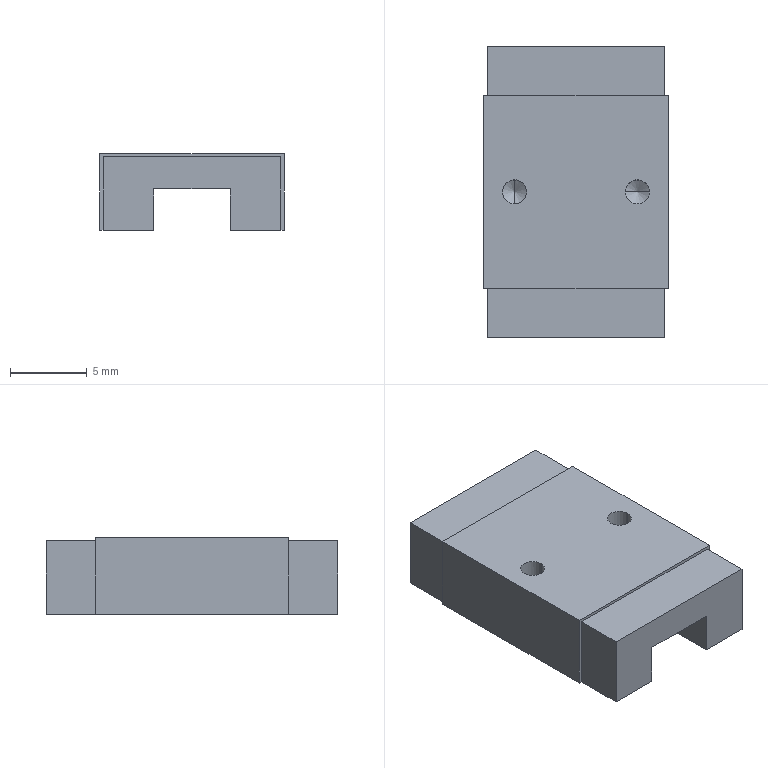Part | SolidWorks | features BaseBody 1 | 1 solid | 26 faces | box 12 x 19 x 5 mm | volume 849.461 mm3 | plane 18 | cylinder 4 | cone 4 | commonest cylinder face diameters 1.567 x4
STEP:
#1=CARTESIAN_POINT('',(-40.025,3.878,3.5));
#2=VERTEX_POINT('',#1);
#3=CARTESIAN_POINT('',(-39.242,3.095,3.5));
#4=VERTEX_POINT('',#3);
#5=CARTESIAN_POINT('',(-39.242,3.878,3.5));
#6=DIRECTION('',(0.,0.,1.));
#7=DIRECTION('',(1.,0.,0.));
#8=AXIS2_PLACEMENT_3D('',#5,#6,#7);
#9=CIRCLE('',#8,0.7835);
#10=EDGE_CURVE('',#2,#4,#9,.T.);
#11=ORIENTED_EDGE('',*,*,#10,.F.);
#12=CARTESIAN_POINT('',(-40.025,3.878,5.));
#13=VERTEX_POINT('',#12);
#14=CARTESIAN_POINT('',(-40.025,3.878,4.25));
#15=DIRECTION('',(0.,0.,1.));
#16=VECTOR('',#15,1000.);
#17=LINE('',#14,#16);
#18=EDGE_CURVE('',#2,#13,#17,.T.);
#19=ORIENTED_EDGE('',*,*,#18,.T.);
#20=CARTESIAN_POINT('',(-38.458,3.878,5.));
#21=VERTEX_POINT('',#20);
#22=CARTESIAN_POINT('',(-39.242,3.878,5.));
#23=DIRECTION('',(0.,0.,-1.));
#24=DIRECTION('',(1.,0.,0.));
#25=AXIS2_PLACEMENT_3D('',#22,#23,#24);
#26=CIRCLE('',#25,0.7835);
#27=EDGE_CURVE('',#21,#13,#26,.T.);
#28=ORIENTED_EDGE('',*,*,#27,.F.);
#29=CARTESIAN_POINT('',(-38.458,3.878,3.5));
#30=VERTEX_POINT('',#29);
#31=CARTESIAN_POINT('',(-38.458,3.878,4.25));
#32=DIRECTION('',(0.,0.,1.));
#33=VECTOR('',#32,1000.);
#34=LINE('',#31,#33);
#35=EDGE_CURVE('',#30,#21,#34,.T.);
#36=ORIENTED_EDGE('',*,*,#35,.F.);
#37=CARTESIAN_POINT('',(-39.242,3.878,3.5));
#38=DIRECTION('',(0.,0.,1.));
#39=DIRECTION('',(1.,0.,0.));
#40=AXIS2_PLACEMENT_3D('',#37,#38,#39);
#41=CIRCLE('',#40,0.7835);
#42=EDGE_CURVE('',#4,#30,#41,.T.);
#43=ORIENTED_EDGE('',*,*,#42,.F.);
#44=EDGE_LOOP('',(#11,#19,#28,#36,#43));
#45=FACE_OUTER_BOUND('',#44,.T.);
#46=CARTESIAN_POINT('',(-39.242,3.878,4.25));
#47=DIRECTION('',(0.,0.,1.));
#48=DIRECTION('',(1.,0.,0.));
#49=AXIS2_PLACEMENT_3D('',#46,#47,#48);
#50=CYLINDRICAL_SURFACE('',#49,0.7835);
#51=ADVANCED_FACE('',(#45),#50,.F.);
#52=CARTESIAN_POINT('',(-32.025,3.878,3.5));
#53=VERTEX_POINT('',#52);
#54=CARTESIAN_POINT('',(-30.458,3.878,3.5));
#55=VERTEX_POINT('',#54);
#56=CARTESIAN_POINT('',(-31.242,3.878,3.5));
#57=DIRECTION('',(0.,0.,1.));
#58=DIRECTION('',(1.,0.,0.));
#59=AXIS2_PLACEMENT_3D('',#56,#57,#58);
#60=CIRCLE('',#59,0.7835);
#61=EDGE_CURVE('',#53,#55,#60,.T.);
#62=ORIENTED_EDGE('',*,*,#61,.F.);
#63=CARTESIAN_POINT('',(-32.025,3.878,5.));
#64=VERTEX_POINT('',#63);
#65=CARTESIAN_POINT('',(-32.025,3.878,4.25));
#66=DIRECTION('',(0.,0.,1.));
#67=VECTOR('',#66,1000.);
#68=LINE('',#65,#67);
#69=EDGE_CURVE('',#53,#64,#68,.T.);
#70=ORIENTED_EDGE('',*,*,#69,.T.);
#71=CARTESIAN_POINT('',(-30.458,3.878,5.));
#72=VERTEX_POINT('',#71);
#73=CARTESIAN_POINT('',(-31.242,3.878,5.));
#74=DIRECTION('',(0.,0.,-1.));
#75=DIRECTION('',(1.,0.,0.));
#76=AXIS2_PLACEMENT_3D('',#73,#74,#75);
#77=CIRCLE('',#76,0.7835);
#78=EDGE_CURVE('',#72,#64,#77,.T.);
#79=ORIENTED_EDGE('',*,*,#78,.F.);
#80=CARTESIAN_POINT('',(-30.458,3.878,4.25));
#81=DIRECTION('',(0.,0.,1.));
#82=VECTOR('',#81,1000.);
#83=LINE('',#80,#82);
#84=EDGE_CURVE('',#55,#72,#83,.T.);
#85=ORIENTED_EDGE('',*,*,#84,.F.);
#86=EDGE_LOOP('',(#62,#70,#79,#85));
#87=FACE_OUTER_BOUND('',#86,.T.);
#88=CARTESIAN_POINT('',(-31.242,3.878,4.25));
#89=DIRECTION('',(0.,0.,1.));
#90=DIRECTION('',(1.,0.,0.));
#91=AXIS2_PLACEMENT_3D('',#88,#89,#90);
#92=CYLINDRICAL_SURFACE('',#91,0.7835);
#93=ADVANCED_FACE('',(#87),#92,.F.);
#94=CARTESIAN_POINT('',(-39.242,3.878,3.029));
#95=VERTEX_POINT('',#94);
#96=CARTESIAN_POINT('',(-39.242,3.095,3.5));
#97=DIRECTION('',(0.,-0.8572,0.515));
#98=VECTOR('',#97,1000.);
#99=LINE('',#96,#98);
#100=EDGE_CURVE('',#95,#4,#99,.T.);
#101=ORIENTED_EDGE('',*,*,#100,.F.);
#102=CARTESIAN_POINT('',(-39.242,4.662,3.5));
#103=VERTEX_POINT('',#102);
#104=CARTESIAN_POINT('',(-39.242,4.662,3.5));
#105=DIRECTION('',(0.,0.8572,0.515));
#106=VECTOR('',#105,1000.);
#107=LINE('',#104,#106);
#108=EDGE_CURVE('',#95,#103,#107,.T.);
#109=ORIENTED_EDGE('',*,*,#108,.T.);
#110=CARTESIAN_POINT('',(-39.242,3.878,3.5));
#111=DIRECTION('',(0.,0.,1.));
#112=DIRECTION('',(1.,0.,0.));
#113=AXIS2_PLACEMENT_3D('',#110,#111,#112);
#114=CIRCLE('',#113,0.7835);
#115=EDGE_CURVE('',#103,#2,#114,.T.);
#116=ORIENTED_EDGE('',*,*,#115,.T.);
#117=ORIENTED_EDGE('',*,*,#10,.T.);
#118=EDGE_LOOP('',(#101,#109,#116,#117));
#119=FACE_OUTER_BOUND('',#118,.T.);
#120=CARTESIAN_POINT('',(-39.242,3.878,3.5));
#121=DIRECTION('',(0.,0.,1.));
#122=DIRECTION('',(0.,-1.,0.));
#123=AXIS2_PLACEMENT_3D('',#120,#121,#122);
#124=CONICAL_SURFACE('',#123,0.7835,1.03);
#125=ADVANCED_FACE('',(#119),#124,.F.);
#126=CARTESIAN_POINT('',(-31.242,3.878,3.029));
#127=VERTEX_POINT('',#126);
#128=CARTESIAN_POINT('',(-30.458,3.878,3.5));
#129=DIRECTION('',(0.8572,0.,0.515));
#130=VECTOR('',#129,1000.);
#131=LINE('',#128,#130);
#132=EDGE_CURVE('',#127,#55,#131,.T.);
#133=ORIENTED_EDGE('',*,*,#132,.F.);
#134=CARTESIAN_POINT('',(-32.025,3.878,3.5));
#135=DIRECTION('',(-0.8572,0.,0.515));
#136=VECTOR('',#135,1000.);
#137=LINE('',#134,#136);
#138=EDGE_CURVE('',#127,#53,#137,.T.);
#139=ORIENTED_EDGE('',*,*,#138,.T.);
#140=ORIENTED_EDGE('',*,*,#61,.T.);
#141=EDGE_LOOP('',(#133,#139,#140));
#142=FACE_OUTER_BOUND('',#141,.T.);
#143=CARTESIAN_POINT('',(-31.242,3.878,3.5));
#144=DIRECTION('',(0.,0.,1.));
#145=DIRECTION('',(1.,0.,0.));
#146=AXIS2_PLACEMENT_3D('',#143,#144,#145);
#147=CONICAL_SURFACE('',#146,0.7835,1.03);
#148=ADVANCED_FACE('',(#142),#147,.F.);
#149=ORIENTED_EDGE('',*,*,#27,.T.);
#150=CARTESIAN_POINT('',(-39.242,3.878,5.));
#151=DIRECTION('',(0.,0.,-1.));
#152=DIRECTION('',(1.,0.,0.));
#153=AXIS2_PLACEMENT_3D('',#150,#151,#152);
#154=CIRCLE('',#153,0.7835);
#155=EDGE_CURVE('',#13,#21,#154,.T.);
#156=ORIENTED_EDGE('',*,*,#155,.T.);
#157=EDGE_LOOP('',(#149,#156));
#158=FACE_BOUND('',#157,.T.);
#159=ORIENTED_EDGE('',*,*,#78,.T.);
#160=CARTESIAN_POINT('',(-31.242,3.878,5.));
#161=DIRECTION('',(0.,0.,-1.));
#162=DIRECTION('',(1.,0.,0.));
#163=AXIS2_PLACEMENT_3D('',#160,#161,#162);
#164=CIRCLE('',#163,0.7835);
#165=EDGE_CURVE('',#64,#72,#164,.T.);
#166=ORIENTED_EDGE('',*,*,#165,.T.);
#167=EDGE_LOOP('',(#159,#166));
#168=FACE_BOUND('',#167,.T.);
#169=CARTESIAN_POINT('',(-41.242,-2.422,5.));
#170=VERTEX_POINT('',#169);
#171=CARTESIAN_POINT('',(-29.242,-2.422,5.));
#172=VERTEX_POINT('',#171);
#173=CARTESIAN_POINT('',(-35.242,-2.422,5.));
#174=DIRECTION('',(1.,0.,0.));
#175=VECTOR('',#174,1000.);
#176=LINE('',#173,#175);
#177=EDGE_CURVE('',#170,#172,#176,.T.);
#178=ORIENTED_EDGE('',*,*,#177,.T.);
#179=CARTESIAN_POINT('',(-29.242,10.178,5.));
#180=VERTEX_POINT('',#179);
#181=CARTESIAN_POINT('',(-29.242,3.878,5.));
#182=DIRECTION('',(0.,1.,0.));
#183=VECTOR('',#182,1000.);
#184=LINE('',#181,#183);
#185=EDGE_CURVE('',#172,#180,#184,.T.);
#186=ORIENTED_EDGE('',*,*,#185,.T.);
#187=CARTESIAN_POINT('',(-41.242,10.178,5.));
#188=VERTEX_POINT('',#187);
#189=CARTESIAN_POINT('',(-35.242,10.178,5.));
#190=DIRECTION('',(-1.,0.,0.));
#191=VECTOR('',#190,1000.);
#192=LINE('',#189,#191);
#193=EDGE_CURVE('',#180,#188,#192,.T.);
#194=ORIENTED_EDGE('',*,*,#193,.T.);
#195=CARTESIAN_POINT('',(-41.242,3.878,5.));
#196=DIRECTION('',(0.,-1.,0.));
#197=VECTOR('',#196,1000.);
#198=LINE('',#195,#197);
#199=EDGE_CURVE('',#188,#170,#198,.T.);
#200=ORIENTED_EDGE('',*,*,#199,.T.);
#201=EDGE_LOOP('',(#178,#186,#194,#200));
#202=FACE_OUTER_BOUND('',#201,.T.);
#203=CARTESIAN_POINT('',(-35.242,3.878,5.));
#204=DIRECTION('',(0.,0.,1.));
#205=DIRECTION('',(1.,0.,0.));
#206=AXIS2_PLACEMENT_3D('',#203,#204,#205);
#207=PLANE('',#206);
#208=ADVANCED_FACE('',(#158,#168,#202),#207,.T.);
#209=ORIENTED_EDGE('',*,*,#18,.F.);
#210=ORIENTED_EDGE('',*,*,#115,.F.);
#211=CARTESIAN_POINT('',(-39.242,3.878,3.5));
#212=DIRECTION('',(0.,0.,1.));
#213=DIRECTION('',(1.,0.,0.));
#214=AXIS2_PLACEMENT_3D('',#211,#212,#213);
#215=CIRCLE('',#214,0.7835);
#216=EDGE_CURVE('',#30,#103,#215,.T.);
#217=ORIENTED_EDGE('',*,*,#216,.F.);
#218=ORIENTED_EDGE('',*,*,#35,.T.);
#219=ORIENTED_EDGE('',*,*,#155,.F.);
#220=EDGE_LOOP('',(#209,#210,#217,#218,#219));
#221=FACE_OUTER_BOUND('',#220,.T.);
#222=CARTESIAN_POINT('',(-39.242,3.878,4.25));
#223=DIRECTION('',(0.,0.,1.));
#224=DIRECTION('',(1.,0.,0.));
#225=AXIS2_PLACEMENT_3D('',#222,#223,#224);
#226=CYLINDRICAL_SURFACE('',#225,0.7835);
#227=ADVANCED_FACE('',(#221),#226,.F.);
#228=ORIENTED_EDGE('',*,*,#69,.F.);
#229=CARTESIAN_POINT('',(-31.242,3.878,3.5));
#230=DIRECTION('',(0.,0.,1.));
#231=DIRECTION('',(1.,0.,0.));
#232=AXIS2_PLACEMENT_3D('',#229,#230,#231);
#233=CIRCLE('',#232,0.7835);
#234=EDGE_CURVE('',#55,#53,#233,.T.);
#235=ORIENTED_EDGE('',*,*,#234,.F.);
#236=ORIENTED_EDGE('',*,*,#84,.T.);
#237=ORIENTED_EDGE('',*,*,#165,.F.);
#238=EDGE_LOOP('',(#228,#235,#236,#237));
#239=FACE_OUTER_BOUND('',#238,.T.);
#240=CARTESIAN_POINT('',(-31.242,3.878,4.25));
#241=DIRECTION('',(0.,0.,1.));
#242=DIRECTION('',(1.,0.,0.));
#243=AXIS2_PLACEMENT_3D('',#240,#241,#242);
#244=CYLINDRICAL_SURFACE('',#243,0.7835);
#245=ADVANCED_FACE('',(#239),#244,.F.);
#246=CARTESIAN_POINT('',(-29.242,10.178,0.));
#247=VERTEX_POINT('',#246);
#248=CARTESIAN_POINT('',(-29.242,10.178,0.));
#249=DIRECTION('',(0.,0.,1.));
#250=VECTOR('',#249,1000.);
#251=LINE('',#248,#250);
#252=EDGE_CURVE('',#247,#180,#251,.T.);
#253=ORIENTED_EDGE('',*,*,#252,.T.);
#254=ORIENTED_EDGE('',*,*,#185,.F.);
#255=CARTESIAN_POINT('',(-29.242,-2.422,0.));
#256=VERTEX_POINT('',#255);
#257=CARTESIAN_POINT('',(-29.242,-2.422,0.));
#258=DIRECTION('',(0.,0.,-1.));
#259=VECTOR('',#258,1000.);
#260=LINE('',#257,#259);
#261=EDGE_CURVE('',#172,#256,#260,.T.);
#262=ORIENTED_EDGE('',*,*,#261,.T.);
#263=CARTESIAN_POINT('',(-29.242,13.378,0.));
#264=DIRECTION('',(0.,1.,0.));
#265=VECTOR('',#264,1000.);
#266=LINE('',#263,#265);
#267=EDGE_CURVE('',#256,#247,#266,.T.);
#268=ORIENTED_EDGE('',*,*,#267,.T.);
#269=EDGE_LOOP('',(#253,#254,#262,#268));
#270=FACE_OUTER_BOUND('',#269,.T.);
#271=CARTESIAN_POINT('',(-29.242,13.378,0.));
#272=DIRECTION('',(1.,0.,0.));
#273=DIRECTION('',(0.,0.,-1.));
#274=AXIS2_PLACEMENT_3D('',#271,#272,#273);
#275=PLANE('',#274);
#276=ADVANCED_FACE('',(#270),#275,.T.);
#277=ORIENTED_EDGE('',*,*,#177,.F.);
#278=CARTESIAN_POINT('',(-41.242,-2.422,0.));
#279=VERTEX_POINT('',#278);
#280=CARTESIAN_POINT('',(-41.242,-2.422,5.));
#281=DIRECTION('',(0.,0.,1.));
#282=VECTOR('',#281,1000.);
#283=LINE('',#280,#282);
#284=EDGE_CURVE('',#279,#170,#283,.T.);
#285=ORIENTED_EDGE('',*,*,#284,.F.);
#286=CARTESIAN_POINT('',(-41.042,-2.422,0.));
#287=VERTEX_POINT('',#286);
#288=CARTESIAN_POINT('',(-35.242,-2.422,0.));
#289=DIRECTION('',(1.,0.,0.));
#290=VECTOR('',#289,1000.);
#291=LINE('',#288,#290);
#292=EDGE_CURVE('',#279,#287,#291,.T.);
#293=ORIENTED_EDGE('',*,*,#292,.T.);
#294=CARTESIAN_POINT('',(-41.042,-2.422,4.8));
#295=VERTEX_POINT('',#294);
#296=CARTESIAN_POINT('',(-41.042,-2.422,5.));
#297=DIRECTION('',(0.,0.,-1.));
#298=VECTOR('',#297,1000.);
#299=LINE('',#296,#298);
#300=EDGE_CURVE('',#295,#287,#299,.T.);
#301=ORIENTED_EDGE('',*,*,#300,.F.);
#302=CARTESIAN_POINT('',(-29.442,-2.422,4.8));
#303=VERTEX_POINT('',#302);
#304=CARTESIAN_POINT('',(-29.242,-2.422,4.8));
#305=DIRECTION('',(-1.,0.,0.));
#306=VECTOR('',#305,1000.);
#307=LINE('',#304,#306);
#308=EDGE_CURVE('',#303,#295,#307,.T.);
#309=ORIENTED_EDGE('',*,*,#308,.F.);
#310=CARTESIAN_POINT('',(-29.442,-2.422,0.));
#311=VERTEX_POINT('',#310);
#312=CARTESIAN_POINT('',(-29.442,-2.422,5.));
#313=DIRECTION('',(0.,0.,1.));
#314=VECTOR('',#313,1000.);
#315=LINE('',#312,#314);
#316=EDGE_CURVE('',#311,#303,#315,.T.);
#317=ORIENTED_EDGE('',*,*,#316,.F.);
#318=CARTESIAN_POINT('',(-29.242,-2.422,0.));
#319=DIRECTION('',(-1.,0.,0.));
#320=VECTOR('',#319,1000.);
#321=LINE('',#318,#320);
#322=EDGE_CURVE('',#256,#311,#321,.T.);
#323=ORIENTED_EDGE('',*,*,#322,.F.);
#324=ORIENTED_EDGE('',*,*,#261,.F.);
#325=EDGE_LOOP('',(#277,#285,#293,#301,#309,#317,#323,#324));
#326=FACE_OUTER_BOUND('',#325,.T.);
#327=CARTESIAN_POINT('',(-29.242,-2.422,5.));
#328=DIRECTION('',(0.,1.,0.));
#329=DIRECTION('',(0.,0.,1.));
#330=AXIS2_PLACEMENT_3D('',#327,#328,#329);
#331=PLANE('',#330);
#332=ADVANCED_FACE('',(#326),#331,.F.);
#333=CARTESIAN_POINT('',(-41.242,10.178,0.));
#334=VERTEX_POINT('',#333);
#335=CARTESIAN_POINT('',(-41.242,10.178,0.));
#336=DIRECTION('',(0.,0.,-1.));
#337=VECTOR('',#336,1000.);
#338=LINE('',#335,#337);
#339=EDGE_CURVE('',#188,#334,#338,.T.);
#340=ORIENTED_EDGE('',*,*,#339,.T.);
#341=CARTESIAN_POINT('',(-41.242,-5.622,0.));
#342=DIRECTION('',(0.,-1.,0.));
#343=VECTOR('',#342,1000.);
#344=LINE('',#341,#343);
#345=EDGE_CURVE('',#334,#279,#344,.T.);
#346=ORIENTED_EDGE('',*,*,#345,.T.);
#347=ORIENTED_EDGE('',*,*,#284,.T.);
#348=ORIENTED_EDGE('',*,*,#199,.F.);
#349=EDGE_LOOP('',(#340,#346,#347,#348));
#350=FACE_OUTER_BOUND('',#349,.T.);
#351=CARTESIAN_POINT('',(-41.242,-5.622,0.));
#352=DIRECTION('',(-1.,0.,0.));
#353=DIRECTION('',(0.,0.,1.));
#354=AXIS2_PLACEMENT_3D('',#351,#352,#353);
#355=PLANE('',#354);
#356=ADVANCED_FACE('',(#350),#355,.T.);
#357=ORIENTED_EDGE('',*,*,#193,.F.);
#358=ORIENTED_EDGE('',*,*,#252,.F.);
#359=CARTESIAN_POINT('',(-29.442,10.178,0.));
#360=VERTEX_POINT('',#359);
#361=CARTESIAN_POINT('',(-41.242,10.178,0.));
#362=DIRECTION('',(1.,0.,0.));
#363=VECTOR('',#362,1000.);
#364=LINE('',#361,#363);
#365=EDGE_CURVE('',#360,#247,#364,.T.);
#366=ORIENTED_EDGE('',*,*,#365,.F.);
#367=CARTESIAN_POINT('',(-29.442,10.178,4.8));
#368=VERTEX_POINT('',#367);
#369=CARTESIAN_POINT('',(-29.442,10.178,5.));
#370=DIRECTION('',(0.,0.,-1.));
#371=VECTOR('',#370,1000.);
#372=LINE('',#369,#371);
#373=EDGE_CURVE('',#368,#360,#372,.T.);
#374=ORIENTED_EDGE('',*,*,#373,.F.);
#375=CARTESIAN_POINT('',(-41.042,10.178,4.8));
#376=VERTEX_POINT('',#375);
#377=CARTESIAN_POINT('',(-41.242,10.178,4.8));
#378=DIRECTION('',(1.,0.,0.));
#379=VECTOR('',#378,1000.);
#380=LINE('',#377,#379);
#381=EDGE_CURVE('',#376,#368,#380,.T.);
#382=ORIENTED_EDGE('',*,*,#381,.F.);
#383=CARTESIAN_POINT('',(-41.042,10.178,0.));
#384=VERTEX_POINT('',#383);
#385=CARTESIAN_POINT('',(-41.042,10.178,5.));
#386=DIRECTION('',(0.,0.,1.));
#387=VECTOR('',#386,1000.);
#388=LINE('',#385,#387);
#389=EDGE_CURVE('',#384,#376,#388,.T.);
#390=ORIENTED_EDGE('',*,*,#389,.F.);
#391=CARTESIAN_POINT('',(-41.242,10.178,0.));
#392=DIRECTION('',(1.,0.,0.));
#393=VECTOR('',#392,1000.);
#394=LINE('',#391,#393);
#395=EDGE_CURVE('',#334,#384,#394,.T.);
#396=ORIENTED_EDGE('',*,*,#395,.F.);
#397=ORIENTED_EDGE('',*,*,#339,.F.);
#398=EDGE_LOOP('',(#357,#358,#366,#374,#382,#390,#396,#397));
#399=FACE_OUTER_BOUND('',#398,.T.);
#400=CARTESIAN_POINT('',(-41.242,10.178,5.));
#401=DIRECTION('',(0.,-1.,0.));
#402=DIRECTION('',(0.,0.,-1.));
#403=AXIS2_PLACEMENT_3D('',#400,#401,#402);
#404=PLANE('',#403);
#405=ADVANCED_FACE('',(#399),#404,.F.);
#406=ORIENTED_EDGE('',*,*,#108,.F.);
#407=ORIENTED_EDGE('',*,*,#100,.T.);
#408=ORIENTED_EDGE('',*,*,#42,.T.);
#409=ORIENTED_EDGE('',*,*,#216,.T.);
#410=EDGE_LOOP('',(#406,#407,#408,#409));
#411=FACE_OUTER_BOUND('',#410,.T.);
#412=CARTESIAN_POINT('',(-39.242,3.878,3.5));
#413=DIRECTION('',(0.,0.,1.));
#414=DIRECTION('',(0.,-1.,0.));
#415=AXIS2_PLACEMENT_3D('',#412,#413,#414);
#416=CONICAL_SURFACE('',#415,0.7835,1.03);
#417=ADVANCED_FACE('',(#411),#416,.F.);
#418=ORIENTED_EDGE('',*,*,#138,.F.);
#419=ORIENTED_EDGE('',*,*,#132,.T.);
#420=ORIENTED_EDGE('',*,*,#234,.T.);
#421=EDGE_LOOP('',(#418,#419,#420));
#422=FACE_OUTER_BOUND('',#421,.T.);
#423=CARTESIAN_POINT('',(-31.242,3.878,3.5));
#424=DIRECTION('',(0.,0.,1.));
#425=DIRECTION('',(1.,0.,0.));
#426=AXIS2_PLACEMENT_3D('',#423,#424,#425);
#427=CONICAL_SURFACE('',#426,0.7835,1.03);
#428=ADVANCED_FACE('',(#422),#427,.F.);
#429=CARTESIAN_POINT('',(-29.442,13.378,0.));
#430=VERTEX_POINT('',#429);
#431=CARTESIAN_POINT('',(-32.742,13.378,0.));
#432=VERTEX_POINT('',#431);
#433=CARTESIAN_POINT('',(-35.242,13.378,0.));
#434=DIRECTION('',(-1.,0.,0.));
#435=VECTOR('',#434,1000.);
#436=LINE('',#433,#435);
#437=EDGE_CURVE('',#430,#432,#436,.T.);
#438=ORIENTED_EDGE('',*,*,#437,.F.);
#439=CARTESIAN_POINT('',(-29.442,3.878,0.));
#440=DIRECTION('',(0.,1.,0.));
#441=VECTOR('',#440,1000.);
#442=LINE('',#439,#441);
#443=EDGE_CURVE('',#360,#430,#442,.T.);
#444=ORIENTED_EDGE('',*,*,#443,.F.);
#445=ORIENTED_EDGE('',*,*,#365,.T.);
#446=ORIENTED_EDGE('',*,*,#267,.F.);
#447=ORIENTED_EDGE('',*,*,#322,.T.);
#448=CARTESIAN_POINT('',(-29.442,-5.622,0.));
#449=VERTEX_POINT('',#448);
#450=CARTESIAN_POINT('',(-29.442,3.878,0.));
#451=DIRECTION('',(0.,1.,0.));
#452=VECTOR('',#451,1000.);
#453=LINE('',#450,#452);
#454=EDGE_CURVE('',#449,#311,#453,.T.);
#455=ORIENTED_EDGE('',*,*,#454,.F.);
#456=CARTESIAN_POINT('',(-32.742,-5.622,0.));
#457=VERTEX_POINT('',#456);
#458=CARTESIAN_POINT('',(-35.242,-5.622,0.));
#459=DIRECTION('',(1.,0.,0.));
#460=VECTOR('',#459,1000.);
#461=LINE('',#458,#460);
#462=EDGE_CURVE('',#457,#449,#461,.T.);
#463=ORIENTED_EDGE('',*,*,#462,.F.);
#464=CARTESIAN_POINT('',(-32.742,3.878,0.));
#465=DIRECTION('',(0.,-1.,0.));
#466=VECTOR('',#465,1000.);
#467=LINE('',#464,#466);
#468=EDGE_CURVE('',#432,#457,#467,.T.);
#469=ORIENTED_EDGE('',*,*,#468,.F.);
#470=EDGE_LOOP('',(#438,#444,#445,#446,#447,#455,#463,#469));
#471=FACE_OUTER_BOUND('',#470,.T.);
#472=CARTESIAN_POINT('',(-35.242,3.878,0.));
#473=DIRECTION('',(0.,0.,1.));
#474=DIRECTION('',(1.,0.,0.));
#475=AXIS2_PLACEMENT_3D('',#472,#473,#474);
#476=PLANE('',#475);
#477=ADVANCED_FACE('',(#471),#476,.F.);
#478=ORIENTED_EDGE('',*,*,#300,.T.);
#479=CARTESIAN_POINT('',(-41.042,-5.622,0.));
#480=VERTEX_POINT('',#479);
#481=CARTESIAN_POINT('',(-41.042,-4.022,0.));
#482=DIRECTION('',(0.,1.,0.));
#483=VECTOR('',#482,1000.);
#484=LINE('',#481,#483);
#485=EDGE_CURVE('',#480,#287,#484,.T.);
#486=ORIENTED_EDGE('',*,*,#485,.F.);
#487=CARTESIAN_POINT('',(-41.042,-5.622,4.8));
#488=VERTEX_POINT('',#487);
#489=CARTESIAN_POINT('',(-41.042,-5.622,2.4));
#490=DIRECTION('',(0.,0.,-1.));
#491=VECTOR('',#490,1000.);
#492=LINE('',#489,#491);
#493=EDGE_CURVE('',#488,#480,#492,.T.);
#494=ORIENTED_EDGE('',*,*,#493,.F.);
#495=CARTESIAN_POINT('',(-41.042,-4.022,4.8));
#496=DIRECTION('',(0.,-1.,0.));
#497=VECTOR('',#496,1000.);
#498=LINE('',#495,#497);
#499=EDGE_CURVE('',#295,#488,#498,.T.);
#500=ORIENTED_EDGE('',*,*,#499,.F.);
#501=EDGE_LOOP('',(#478,#486,#494,#500));
#502=FACE_OUTER_BOUND('',#501,.T.);
#503=CARTESIAN_POINT('',(-41.042,-4.022,2.4));
#504=DIRECTION('',(1.,0.,0.));
#505=DIRECTION('',(0.,0.,-1.));
#506=AXIS2_PLACEMENT_3D('',#503,#504,#505);
#507=PLANE('',#506);
#508=ADVANCED_FACE('',(#502),#507,.F.);
#509=CARTESIAN_POINT('',(-29.442,-5.622,4.8));
#510=VERTEX_POINT('',#509);
#511=CARTESIAN_POINT('',(-29.442,-4.022,4.8));
#512=DIRECTION('',(0.,1.,0.));
#513=VECTOR('',#512,1000.);
#514=LINE('',#511,#513);
#515=EDGE_CURVE('',#510,#303,#514,.T.);
#516=ORIENTED_EDGE('',*,*,#515,.T.);
#517=ORIENTED_EDGE('',*,*,#308,.T.);
#518=ORIENTED_EDGE('',*,*,#499,.T.);
#519=CARTESIAN_POINT('',(-35.242,-5.622,4.8));
#520=DIRECTION('',(1.,0.,0.));
#521=VECTOR('',#520,1000.);
#522=LINE('',#519,#521);
#523=EDGE_CURVE('',#488,#510,#522,.T.);
#524=ORIENTED_EDGE('',*,*,#523,.T.);
#525=EDGE_LOOP('',(#516,#517,#518,#524));
#526=FACE_OUTER_BOUND('',#525,.T.);
#527=CARTESIAN_POINT('',(-35.242,-4.022,4.8));
#528=DIRECTION('',(0.,0.,1.));
#529=DIRECTION('',(1.,0.,0.));
#530=AXIS2_PLACEMENT_3D('',#527,#528,#529);
#531=PLANE('',#530);
#532=ADVANCED_FACE('',(#526),#531,.T.);
#533=ORIENTED_EDGE('',*,*,#316,.T.);
#534=ORIENTED_EDGE('',*,*,#515,.F.);
#535=CARTESIAN_POINT('',(-29.442,-5.622,2.4));
#536=DIRECTION('',(0.,0.,-1.));
#537=VECTOR('',#536,1000.);
#538=LINE('',#535,#537);
#539=EDGE_CURVE('',#510,#449,#538,.T.);
#540=ORIENTED_EDGE('',*,*,#539,.T.);
#541=ORIENTED_EDGE('',*,*,#454,.T.);
#542=EDGE_LOOP('',(#533,#534,#540,#541));
#543=FACE_OUTER_BOUND('',#542,.T.);
#544=CARTESIAN_POINT('',(-29.442,-4.022,2.4));
#545=DIRECTION('',(1.,0.,0.));
#546=DIRECTION('',(0.,0.,-1.));
#547=AXIS2_PLACEMENT_3D('',#544,#545,#546);
#548=PLANE('',#547);
#549=ADVANCED_FACE('',(#543),#548,.T.);
#550=CARTESIAN_POINT('',(-37.742,-5.622,0.));
#551=VERTEX_POINT('',#550);
#552=CARTESIAN_POINT('',(-35.242,-5.622,0.));
#553=DIRECTION('',(1.,0.,0.));
#554=VECTOR('',#553,1000.);
#555=LINE('',#552,#554);
#556=EDGE_CURVE('',#480,#551,#555,.T.);
#557=ORIENTED_EDGE('',*,*,#556,.F.);
#558=ORIENTED_EDGE('',*,*,#485,.T.);
#559=ORIENTED_EDGE('',*,*,#292,.F.);
#560=ORIENTED_EDGE('',*,*,#345,.F.);
#561=ORIENTED_EDGE('',*,*,#395,.T.);
#562=CARTESIAN_POINT('',(-41.042,13.378,0.));
#563=VERTEX_POINT('',#562);
#564=CARTESIAN_POINT('',(-41.042,3.878,0.));
#565=DIRECTION('',(0.,-1.,0.));
#566=VECTOR('',#565,1000.);
#567=LINE('',#564,#566);
#568=EDGE_CURVE('',#563,#384,#567,.T.);
#569=ORIENTED_EDGE('',*,*,#568,.F.);
#570=CARTESIAN_POINT('',(-37.742,13.378,0.));
#571=VERTEX_POINT('',#570);
#572=CARTESIAN_POINT('',(-35.242,13.378,0.));
#573=DIRECTION('',(-1.,0.,0.));
#574=VECTOR('',#573,1000.);
#575=LINE('',#572,#574);
#576=EDGE_CURVE('',#571,#563,#575,.T.);
#577=ORIENTED_EDGE('',*,*,#576,.F.);
#578=CARTESIAN_POINT('',(-37.742,3.878,0.));
#579=DIRECTION('',(0.,1.,0.));
#580=VECTOR('',#579,1000.);
#581=LINE('',#578,#580);
#582=EDGE_CURVE('',#551,#571,#581,.T.);
#583=ORIENTED_EDGE('',*,*,#582,.F.);
#584=EDGE_LOOP('',(#557,#558,#559,#560,#561,#569,#577,#583));
#585=FACE_OUTER_BOUND('',#584,.T.);
#586=CARTESIAN_POINT('',(-35.242,3.878,0.));
#587=DIRECTION('',(0.,0.,1.));
#588=DIRECTION('',(1.,0.,0.));
#589=AXIS2_PLACEMENT_3D('',#586,#587,#588);
#590=PLANE('',#589);
#591=ADVANCED_FACE('',(#585),#590,.F.);
#592=CARTESIAN_POINT('',(-29.442,13.378,4.8));
#593=VERTEX_POINT('',#592);
#594=CARTESIAN_POINT('',(-29.442,11.778,4.8));
#595=DIRECTION('',(0.,-1.,0.));
#596=VECTOR('',#595,1000.);
#597=LINE('',#594,#596);
#598=EDGE_CURVE('',#593,#368,#597,.T.);
#599=ORIENTED_EDGE('',*,*,#598,.T.);
#600=ORIENTED_EDGE('',*,*,#373,.T.);
#601=ORIENTED_EDGE('',*,*,#443,.T.);
#602=CARTESIAN_POINT('',(-29.442,13.378,2.4));
#603=DIRECTION('',(0.,0.,1.));
#604=VECTOR('',#603,1000.);
#605=LINE('',#602,#604);
#606=EDGE_CURVE('',#430,#593,#605,.T.);
#607=ORIENTED_EDGE('',*,*,#606,.T.);
#608=EDGE_LOOP('',(#599,#600,#601,#607));
#609=FACE_OUTER_BOUND('',#608,.T.);
#610=CARTESIAN_POINT('',(-29.442,11.778,2.4));
#611=DIRECTION('',(1.,0.,0.));
#612=DIRECTION('',(0.,0.,-1.));
#613=AXIS2_PLACEMENT_3D('',#610,#611,#612);
#614=PLANE('',#613);
#615=ADVANCED_FACE('',(#609),#614,.T.);
#616=ORIENTED_EDGE('',*,*,#598,.F.);
#617=CARTESIAN_POINT('',(-41.042,13.378,4.8));
#618=VERTEX_POINT('',#617);
#619=CARTESIAN_POINT('',(-35.242,13.378,4.8));
#620=DIRECTION('',(-1.,0.,0.));
#621=VECTOR('',#620,1000.);
#622=LINE('',#619,#621);
#623=EDGE_CURVE('',#593,#618,#622,.T.);
#624=ORIENTED_EDGE('',*,*,#623,.T.);
#625=CARTESIAN_POINT('',(-41.042,11.778,4.8));
#626=DIRECTION('',(0.,-1.,0.));
#627=VECTOR('',#626,1000.);
#628=LINE('',#625,#627);
#629=EDGE_CURVE('',#618,#376,#628,.T.);
#630=ORIENTED_EDGE('',*,*,#629,.T.);
#631=ORIENTED_EDGE('',*,*,#381,.T.);
#632=EDGE_LOOP('',(#616,#624,#630,#631));
#633=FACE_OUTER_BOUND('',#632,.T.);
#634=CARTESIAN_POINT('',(-35.242,11.778,4.8));
#635=DIRECTION('',(0.,0.,1.));
#636=DIRECTION('',(1.,0.,0.));
#637=AXIS2_PLACEMENT_3D('',#634,#635,#636);
#638=PLANE('',#637);
#639=ADVANCED_FACE('',(#633),#638,.T.);
#640=ORIENTED_EDGE('',*,*,#568,.T.);
#641=ORIENTED_EDGE('',*,*,#389,.T.);
#642=ORIENTED_EDGE('',*,*,#629,.F.);
#643=CARTESIAN_POINT('',(-41.042,13.378,2.4));
#644=DIRECTION('',(0.,0.,1.));
#645=VECTOR('',#644,1000.);
#646=LINE('',#643,#645);
#647=EDGE_CURVE('',#563,#618,#646,.T.);
#648=ORIENTED_EDGE('',*,*,#647,.F.);
#649=EDGE_LOOP('',(#640,#641,#642,#648));
#650=FACE_OUTER_BOUND('',#649,.T.);
#651=CARTESIAN_POINT('',(-41.042,11.778,2.4));
#652=DIRECTION('',(1.,0.,0.));
#653=DIRECTION('',(0.,0.,-1.));
#654=AXIS2_PLACEMENT_3D('',#651,#652,#653);
#655=PLANE('',#654);
#656=ADVANCED_FACE('',(#650),#655,.F.);
#657=CARTESIAN_POINT('',(-32.742,13.378,2.7));
#658=VERTEX_POINT('',#657);
#659=CARTESIAN_POINT('',(-32.742,13.378,0.));
#660=DIRECTION('',(0.,0.,1.));
#661=VECTOR('',#660,1000.);
#662=LINE('',#659,#661);
#663=EDGE_CURVE('',#432,#658,#662,.T.);
#664=ORIENTED_EDGE('',*,*,#663,.F.);
#665=ORIENTED_EDGE('',*,*,#468,.T.);
#666=CARTESIAN_POINT('',(-32.742,-5.622,2.7));
#667=VERTEX_POINT('',#666);
#668=CARTESIAN_POINT('',(-32.742,-5.622,0.));
#669=DIRECTION('',(0.,0.,-1.));
#670=VECTOR('',#669,1000.);
#671=LINE('',#668,#670);
#672=EDGE_CURVE('',#667,#457,#671,.T.);
#673=ORIENTED_EDGE('',*,*,#672,.F.);
#674=CARTESIAN_POINT('',(-32.742,13.378,2.7));
#675=DIRECTION('',(0.,-1.,0.));
#676=VECTOR('',#675,1000.);
#677=LINE('',#674,#676);
#678=EDGE_CURVE('',#658,#667,#677,.T.);
#679=ORIENTED_EDGE('',*,*,#678,.F.);
#680=EDGE_LOOP('',(#664,#665,#673,#679));
#681=FACE_OUTER_BOUND('',#680,.T.);
#682=CARTESIAN_POINT('',(-32.742,13.378,0.));
#683=DIRECTION('',(1.,0.,0.));
#684=DIRECTION('',(0.,0.,-1.));
#685=AXIS2_PLACEMENT_3D('',#682,#683,#684);
#686=PLANE('',#685);
#687=ADVANCED_FACE('',(#681),#686,.F.);
#688=ORIENTED_EDGE('',*,*,#606,.F.);
#689=ORIENTED_EDGE('',*,*,#437,.T.);
#690=ORIENTED_EDGE('',*,*,#663,.T.);
#691=CARTESIAN_POINT('',(-37.742,13.378,2.7));
#692=VERTEX_POINT('',#691);
#693=CARTESIAN_POINT('',(-41.242,13.378,2.7));
#694=DIRECTION('',(-1.,0.,0.));
#695=VECTOR('',#694,1000.);
#696=LINE('',#693,#695);
#697=EDGE_CURVE('',#658,#692,#696,.T.);
#698=ORIENTED_EDGE('',*,*,#697,.T.);
#699=CARTESIAN_POINT('',(-37.742,13.378,0.));
#700=DIRECTION('',(0.,0.,-1.));
#701=VECTOR('',#700,1000.);
#702=LINE('',#699,#701);
#703=EDGE_CURVE('',#692,#571,#702,.T.);
#704=ORIENTED_EDGE('',*,*,#703,.T.);
#705=ORIENTED_EDGE('',*,*,#576,.T.);
#706=ORIENTED_EDGE('',*,*,#647,.T.);
#707=ORIENTED_EDGE('',*,*,#623,.F.);
#708=EDGE_LOOP('',(#688,#689,#690,#698,#704,#705,#706,#707));
#709=FACE_OUTER_BOUND('',#708,.T.);
#710=CARTESIAN_POINT('',(-41.242,13.378,0.));
#711=DIRECTION('',(0.,1.,0.));
#712=DIRECTION('',(0.,0.,1.));
#713=AXIS2_PLACEMENT_3D('',#710,#711,#712);
#714=PLANE('',#713);
#715=ADVANCED_FACE('',(#709),#714,.T.);
#716=CARTESIAN_POINT('',(-37.742,-5.622,2.7));
#717=VERTEX_POINT('',#716);
#718=CARTESIAN_POINT('',(-37.742,-5.622,0.));
#719=DIRECTION('',(0.,0.,1.));
#720=VECTOR('',#719,1000.);
#721=LINE('',#718,#720);
#722=EDGE_CURVE('',#551,#717,#721,.T.);
#723=ORIENTED_EDGE('',*,*,#722,.T.);
#724=CARTESIAN_POINT('',(-29.242,-5.622,2.7));
#725=DIRECTION('',(1.,0.,0.));
#726=VECTOR('',#725,1000.);
#727=LINE('',#724,#726);
#728=EDGE_CURVE('',#717,#667,#727,.T.);
#729=ORIENTED_EDGE('',*,*,#728,.T.);
#730=ORIENTED_EDGE('',*,*,#672,.T.);
#731=ORIENTED_EDGE('',*,*,#462,.T.);
#732=ORIENTED_EDGE('',*,*,#539,.F.);
#733=ORIENTED_EDGE('',*,*,#523,.F.);
#734=ORIENTED_EDGE('',*,*,#493,.T.);
#735=ORIENTED_EDGE('',*,*,#556,.T.);
#736=EDGE_LOOP('',(#723,#729,#730,#731,#732,#733,#734,#735));
#737=FACE_OUTER_BOUND('',#736,.T.);
#738=CARTESIAN_POINT('',(-29.242,-5.622,0.));
#739=DIRECTION('',(0.,-1.,0.));
#740=DIRECTION('',(0.,0.,-1.));
#741=AXIS2_PLACEMENT_3D('',#738,#739,#740);
#742=PLANE('',#741);
#743=ADVANCED_FACE('',(#737),#742,.T.);
#744=ORIENTED_EDGE('',*,*,#722,.F.);
#745=ORIENTED_EDGE('',*,*,#582,.T.);
#746=ORIENTED_EDGE('',*,*,#703,.F.);
#747=CARTESIAN_POINT('',(-37.742,-5.622,2.7));
#748=DIRECTION('',(0.,1.,0.));
#749=VECTOR('',#748,1000.);
#750=LINE('',#747,#749);
#751=EDGE_CURVE('',#717,#692,#750,.T.);
#752=ORIENTED_EDGE('',*,*,#751,.F.);
#753=EDGE_LOOP('',(#744,#745,#746,#752));
#754=FACE_OUTER_BOUND('',#753,.T.);
#755=CARTESIAN_POINT('',(-37.742,-5.622,0.));
#756=DIRECTION('',(-1.,0.,0.));
#757=DIRECTION('',(0.,0.,1.));
#758=AXIS2_PLACEMENT_3D('',#755,#756,#757);
#759=PLANE('',#758);
#760=ADVANCED_FACE('',(#754),#759,.F.);
#761=ORIENTED_EDGE('',*,*,#751,.T.);
#762=ORIENTED_EDGE('',*,*,#697,.F.);
#763=ORIENTED_EDGE('',*,*,#678,.T.);
#764=ORIENTED_EDGE('',*,*,#728,.F.);
#765=EDGE_LOOP('',(#761,#762,#763,#764));
#766=FACE_OUTER_BOUND('',#765,.T.);
#767=CARTESIAN_POINT('',(-35.242,3.878,2.7));
#768=DIRECTION('',(0.,0.,1.));
#769=DIRECTION('',(1.,0.,0.));
#770=AXIS2_PLACEMENT_3D('',#767,#768,#769);
#771=PLANE('',#770);
#772=ADVANCED_FACE('',(#766),#771,.F.);
#773=CLOSED_SHELL('',(#51,#93,#125,#148,#208,#227,#245,#276,#332,#356,#405,#417,#428,#477,#508,#532,#549,#591,#615,#639,#656,#687,#715,#743,#760,#772));
#774=MANIFOLD_SOLID_BREP('',#773);
#775=CARTESIAN_POINT('',(0.,0.,0.));
#776=DIRECTION('',(0.,0.,1.));
#777=DIRECTION('',(1.,0.,0.));
#778=AXIS2_PLACEMENT_3D('',#775,#776,#777);
#779=(LENGTH_UNIT()NAMED_UNIT(*)SI_UNIT(.MILLI.,.METRE.));
#780=UNCERTAINTY_MEASURE_WITH_UNIT(LENGTH_MEASURE(0.00001),#779,'','');
#781=(NAMED_UNIT(*)PLANE_ANGLE_UNIT()SI_UNIT($,.RADIAN.));
#782=(NAMED_UNIT(*)SI_UNIT($,.STERADIAN.)SOLID_ANGLE_UNIT());
#783=(GEOMETRIC_REPRESENTATION_CONTEXT(3)GLOBAL_UNCERTAINTY_ASSIGNED_CONTEXT((#780))GLOBAL_UNIT_ASSIGNED_CONTEXT((#779,#781,#782))REPRESENTATION_CONTEXT('',''));
#784=ADVANCED_BREP_SHAPE_REPRESENTATION('',(#774,#778),#783);